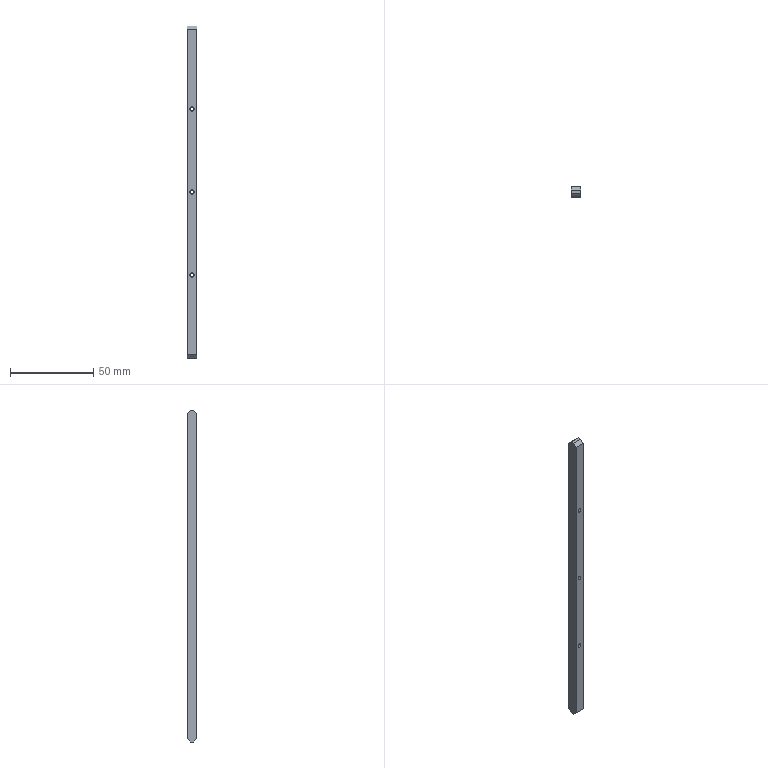Part | SolidWorks | features 3DProfileFeature 1, Chamfer 1, Extrusion 1, HoleWzd 1 | 1 solid | 16 faces | box 6 x 6 x 200 mm | volume 7064 mm3 | plane 10 | cylinder 6 | commonest cylinder face diameters 2.5 x6
STEP:
#1=CARTESIAN_POINT('',(0.,-3.,48.75));
#2=VERTEX_POINT('',#1);
#3=CARTESIAN_POINT('',(0.,-3.,51.25));
#4=VERTEX_POINT('',#3);
#5=CARTESIAN_POINT('',(0.,-3.,50.));
#6=DIRECTION('',(0.,1.,0.));
#7=DIRECTION('',(0.,0.,1.));
#8=AXIS2_PLACEMENT_3D('',#5,#6,#7);
#9=CIRCLE('',#8,1.25);
#10=EDGE_CURVE('',#2,#4,#9,.T.);
#11=ORIENTED_EDGE('',*,*,#10,.F.);
#12=CARTESIAN_POINT('',(0.,3.,48.75));
#13=VERTEX_POINT('',#12);
#14=CARTESIAN_POINT('',(0.,3.,48.75));
#15=DIRECTION('',(0.,1.,0.));
#16=VECTOR('',#15,1000.);
#17=LINE('',#14,#16);
#18=EDGE_CURVE('',#2,#13,#17,.T.);
#19=ORIENTED_EDGE('',*,*,#18,.T.);
#20=CARTESIAN_POINT('',(0.,3.,51.25));
#21=VERTEX_POINT('',#20);
#22=CARTESIAN_POINT('',(0.,3.,50.));
#23=DIRECTION('',(0.,1.,0.));
#24=DIRECTION('',(0.,0.,1.));
#25=AXIS2_PLACEMENT_3D('',#22,#23,#24);
#26=CIRCLE('',#25,1.25);
#27=EDGE_CURVE('',#13,#21,#26,.T.);
#28=ORIENTED_EDGE('',*,*,#27,.T.);
#29=CARTESIAN_POINT('',(0.,3.,51.25));
#30=DIRECTION('',(0.,1.,0.));
#31=VECTOR('',#30,1000.);
#32=LINE('',#29,#31);
#33=EDGE_CURVE('',#4,#21,#32,.T.);
#34=ORIENTED_EDGE('',*,*,#33,.F.);
#35=EDGE_LOOP('',(#11,#19,#28,#34));
#36=FACE_OUTER_BOUND('',#35,.T.);
#37=CARTESIAN_POINT('',(0.,3.,50.));
#38=DIRECTION('',(0.,1.,0.));
#39=DIRECTION('',(0.,0.,1.));
#40=AXIS2_PLACEMENT_3D('',#37,#38,#39);
#41=CYLINDRICAL_SURFACE('',#40,1.25);
#42=ADVANCED_FACE('',(#36),#41,.F.);
#43=CARTESIAN_POINT('',(0.,-3.,98.75));
#44=VERTEX_POINT('',#43);
#45=CARTESIAN_POINT('',(0.,-3.,101.25));
#46=VERTEX_POINT('',#45);
#47=CARTESIAN_POINT('',(0.,-3.,100.));
#48=DIRECTION('',(0.,1.,0.));
#49=DIRECTION('',(0.,0.,1.));
#50=AXIS2_PLACEMENT_3D('',#47,#48,#49);
#51=CIRCLE('',#50,1.25);
#52=EDGE_CURVE('',#44,#46,#51,.T.);
#53=ORIENTED_EDGE('',*,*,#52,.F.);
#54=CARTESIAN_POINT('',(0.,3.,98.75));
#55=VERTEX_POINT('',#54);
#56=CARTESIAN_POINT('',(0.,3.,98.75));
#57=DIRECTION('',(0.,1.,0.));
#58=VECTOR('',#57,1000.);
#59=LINE('',#56,#58);
#60=EDGE_CURVE('',#44,#55,#59,.T.);
#61=ORIENTED_EDGE('',*,*,#60,.T.);
#62=CARTESIAN_POINT('',(0.,3.,101.25));
#63=VERTEX_POINT('',#62);
#64=CARTESIAN_POINT('',(0.,3.,100.));
#65=DIRECTION('',(0.,1.,0.));
#66=DIRECTION('',(0.,0.,1.));
#67=AXIS2_PLACEMENT_3D('',#64,#65,#66);
#68=CIRCLE('',#67,1.25);
#69=EDGE_CURVE('',#55,#63,#68,.T.);
#70=ORIENTED_EDGE('',*,*,#69,.T.);
#71=CARTESIAN_POINT('',(0.,3.,101.25));
#72=DIRECTION('',(0.,1.,0.));
#73=VECTOR('',#72,1000.);
#74=LINE('',#71,#73);
#75=EDGE_CURVE('',#46,#63,#74,.T.);
#76=ORIENTED_EDGE('',*,*,#75,.F.);
#77=EDGE_LOOP('',(#53,#61,#70,#76));
#78=FACE_OUTER_BOUND('',#77,.T.);
#79=CARTESIAN_POINT('',(0.,3.,100.));
#80=DIRECTION('',(0.,1.,0.));
#81=DIRECTION('',(0.,0.,1.));
#82=AXIS2_PLACEMENT_3D('',#79,#80,#81);
#83=CYLINDRICAL_SURFACE('',#82,1.25);
#84=ADVANCED_FACE('',(#78),#83,.F.);
#85=CARTESIAN_POINT('',(0.,-3.,148.75));
#86=VERTEX_POINT('',#85);
#87=CARTESIAN_POINT('',(0.,-3.,151.25));
#88=VERTEX_POINT('',#87);
#89=CARTESIAN_POINT('',(0.,-3.,150.));
#90=DIRECTION('',(0.,1.,0.));
#91=DIRECTION('',(0.,0.,1.));
#92=AXIS2_PLACEMENT_3D('',#89,#90,#91);
#93=CIRCLE('',#92,1.25);
#94=EDGE_CURVE('',#86,#88,#93,.T.);
#95=ORIENTED_EDGE('',*,*,#94,.F.);
#96=CARTESIAN_POINT('',(0.,3.,148.75));
#97=VERTEX_POINT('',#96);
#98=CARTESIAN_POINT('',(0.,3.,148.75));
#99=DIRECTION('',(0.,1.,0.));
#100=VECTOR('',#99,1000.);
#101=LINE('',#98,#100);
#102=EDGE_CURVE('',#86,#97,#101,.T.);
#103=ORIENTED_EDGE('',*,*,#102,.T.);
#104=CARTESIAN_POINT('',(0.,3.,151.25));
#105=VERTEX_POINT('',#104);
#106=CARTESIAN_POINT('',(0.,3.,150.));
#107=DIRECTION('',(0.,1.,0.));
#108=DIRECTION('',(0.,0.,1.));
#109=AXIS2_PLACEMENT_3D('',#106,#107,#108);
#110=CIRCLE('',#109,1.25);
#111=EDGE_CURVE('',#97,#105,#110,.T.);
#112=ORIENTED_EDGE('',*,*,#111,.T.);
#113=CARTESIAN_POINT('',(0.,3.,151.25));
#114=DIRECTION('',(0.,1.,0.));
#115=VECTOR('',#114,1000.);
#116=LINE('',#113,#115);
#117=EDGE_CURVE('',#88,#105,#116,.T.);
#118=ORIENTED_EDGE('',*,*,#117,.F.);
#119=EDGE_LOOP('',(#95,#103,#112,#118));
#120=FACE_OUTER_BOUND('',#119,.T.);
#121=CARTESIAN_POINT('',(0.,3.,150.));
#122=DIRECTION('',(0.,1.,0.));
#123=DIRECTION('',(0.,0.,1.));
#124=AXIS2_PLACEMENT_3D('',#121,#122,#123);
#125=CYLINDRICAL_SURFACE('',#124,1.25);
#126=ADVANCED_FACE('',(#120),#125,.F.);
#127=CARTESIAN_POINT('',(3.,-3.,198.));
#128=VERTEX_POINT('',#127);
#129=CARTESIAN_POINT('',(3.,-3.,2.));
#130=VERTEX_POINT('',#129);
#131=CARTESIAN_POINT('',(3.,-3.,200.));
#132=DIRECTION('',(0.,0.,-1.));
#133=VECTOR('',#132,1000.);
#134=LINE('',#131,#133);
#135=EDGE_CURVE('',#128,#130,#134,.T.);
#136=ORIENTED_EDGE('',*,*,#135,.T.);
#137=CARTESIAN_POINT('',(3.,-1.,0.));
#138=VERTEX_POINT('',#137);
#139=CARTESIAN_POINT('',(3.,-3.,2.));
#140=DIRECTION('',(0.,0.7071,-0.7071));
#141=VECTOR('',#140,1000.);
#142=LINE('',#139,#141);
#143=EDGE_CURVE('',#130,#138,#142,.T.);
#144=ORIENTED_EDGE('',*,*,#143,.T.);
#145=CARTESIAN_POINT('',(3.,1.,0.));
#146=VERTEX_POINT('',#145);
#147=CARTESIAN_POINT('',(3.,3.,0.));
#148=DIRECTION('',(0.,1.,0.));
#149=VECTOR('',#148,1000.);
#150=LINE('',#147,#149);
#151=EDGE_CURVE('',#138,#146,#150,.T.);
#152=ORIENTED_EDGE('',*,*,#151,.T.);
#153=CARTESIAN_POINT('',(3.,3.,2.));
#154=VERTEX_POINT('',#153);
#155=CARTESIAN_POINT('',(3.,3.,2.));
#156=DIRECTION('',(0.,0.7071,0.7071));
#157=VECTOR('',#156,1000.);
#158=LINE('',#155,#157);
#159=EDGE_CURVE('',#146,#154,#158,.T.);
#160=ORIENTED_EDGE('',*,*,#159,.T.);
#161=CARTESIAN_POINT('',(3.,3.,198.));
#162=VERTEX_POINT('',#161);
#163=CARTESIAN_POINT('',(3.,3.,200.));
#164=DIRECTION('',(0.,0.,-1.));
#165=VECTOR('',#164,1000.);
#166=LINE('',#163,#165);
#167=EDGE_CURVE('',#162,#154,#166,.T.);
#168=ORIENTED_EDGE('',*,*,#167,.F.);
#169=CARTESIAN_POINT('',(3.,1.,200.));
#170=VERTEX_POINT('',#169);
#171=CARTESIAN_POINT('',(3.,1.,200.));
#172=DIRECTION('',(0.,-0.7071,0.7071));
#173=VECTOR('',#172,1000.);
#174=LINE('',#171,#173);
#175=EDGE_CURVE('',#162,#170,#174,.T.);
#176=ORIENTED_EDGE('',*,*,#175,.T.);
#177=CARTESIAN_POINT('',(3.,-1.,200.));
#178=VERTEX_POINT('',#177);
#179=CARTESIAN_POINT('',(3.,3.,200.));
#180=DIRECTION('',(0.,1.,0.));
#181=VECTOR('',#180,1000.);
#182=LINE('',#179,#181);
#183=EDGE_CURVE('',#178,#170,#182,.T.);
#184=ORIENTED_EDGE('',*,*,#183,.F.);
#185=CARTESIAN_POINT('',(3.,-1.,200.));
#186=DIRECTION('',(0.,-0.7071,-0.7071));
#187=VECTOR('',#186,1000.);
#188=LINE('',#185,#187);
#189=EDGE_CURVE('',#178,#128,#188,.T.);
#190=ORIENTED_EDGE('',*,*,#189,.T.);
#191=EDGE_LOOP('',(#136,#144,#152,#160,#168,#176,#184,#190));
#192=FACE_OUTER_BOUND('',#191,.T.);
#193=CARTESIAN_POINT('',(3.,3.,200.));
#194=DIRECTION('',(-1.,0.,0.));
#195=DIRECTION('',(0.,-1.,0.));
#196=AXIS2_PLACEMENT_3D('',#193,#194,#195);
#197=PLANE('',#196);
#198=ADVANCED_FACE('',(#192),#197,.F.);
#199=CARTESIAN_POINT('',(0.,3.,50.));
#200=DIRECTION('',(0.,1.,0.));
#201=DIRECTION('',(0.,0.,1.));
#202=AXIS2_PLACEMENT_3D('',#199,#200,#201);
#203=CIRCLE('',#202,1.25);
#204=EDGE_CURVE('',#21,#13,#203,.T.);
#205=ORIENTED_EDGE('',*,*,#204,.F.);
#206=ORIENTED_EDGE('',*,*,#27,.F.);
#207=EDGE_LOOP('',(#205,#206));
#208=FACE_BOUND('',#207,.T.);
#209=CARTESIAN_POINT('',(0.,3.,100.));
#210=DIRECTION('',(0.,1.,0.));
#211=DIRECTION('',(0.,0.,1.));
#212=AXIS2_PLACEMENT_3D('',#209,#210,#211);
#213=CIRCLE('',#212,1.25);
#214=EDGE_CURVE('',#63,#55,#213,.T.);
#215=ORIENTED_EDGE('',*,*,#214,.F.);
#216=ORIENTED_EDGE('',*,*,#69,.F.);
#217=EDGE_LOOP('',(#215,#216));
#218=FACE_BOUND('',#217,.T.);
#219=CARTESIAN_POINT('',(0.,3.,150.));
#220=DIRECTION('',(0.,1.,0.));
#221=DIRECTION('',(0.,0.,1.));
#222=AXIS2_PLACEMENT_3D('',#219,#220,#221);
#223=CIRCLE('',#222,1.25);
#224=EDGE_CURVE('',#105,#97,#223,.T.);
#225=ORIENTED_EDGE('',*,*,#224,.F.);
#226=ORIENTED_EDGE('',*,*,#111,.F.);
#227=EDGE_LOOP('',(#225,#226));
#228=FACE_BOUND('',#227,.T.);
#229=ORIENTED_EDGE('',*,*,#167,.T.);
#230=CARTESIAN_POINT('',(-3.,3.,2.));
#231=VERTEX_POINT('',#230);
#232=CARTESIAN_POINT('',(-3.,3.,2.));
#233=DIRECTION('',(-1.,0.,0.));
#234=VECTOR('',#233,1000.);
#235=LINE('',#232,#234);
#236=EDGE_CURVE('',#154,#231,#235,.T.);
#237=ORIENTED_EDGE('',*,*,#236,.T.);
#238=CARTESIAN_POINT('',(-3.,3.,198.));
#239=VERTEX_POINT('',#238);
#240=CARTESIAN_POINT('',(-3.,3.,200.));
#241=DIRECTION('',(0.,0.,-1.));
#242=VECTOR('',#241,1000.);
#243=LINE('',#240,#242);
#244=EDGE_CURVE('',#239,#231,#243,.T.);
#245=ORIENTED_EDGE('',*,*,#244,.F.);
#246=CARTESIAN_POINT('',(3.,3.,198.));
#247=DIRECTION('',(1.,0.,0.));
#248=VECTOR('',#247,1000.);
#249=LINE('',#246,#248);
#250=EDGE_CURVE('',#239,#162,#249,.T.);
#251=ORIENTED_EDGE('',*,*,#250,.T.);
#252=EDGE_LOOP('',(#229,#237,#245,#251));
#253=FACE_OUTER_BOUND('',#252,.T.);
#254=CARTESIAN_POINT('',(-3.,3.,200.));
#255=DIRECTION('',(0.,-1.,0.));
#256=DIRECTION('',(0.,0.,-1.));
#257=AXIS2_PLACEMENT_3D('',#254,#255,#256);
#258=PLANE('',#257);
#259=ADVANCED_FACE('',(#208,#218,#228,#253),#258,.F.);
#260=CARTESIAN_POINT('',(-3.,1.,0.));
#261=VERTEX_POINT('',#260);
#262=CARTESIAN_POINT('',(-3.,-1.,0.));
#263=VERTEX_POINT('',#262);
#264=CARTESIAN_POINT('',(-3.,3.,0.));
#265=DIRECTION('',(0.,-1.,0.));
#266=VECTOR('',#265,1000.);
#267=LINE('',#264,#266);
#268=EDGE_CURVE('',#261,#263,#267,.T.);
#269=ORIENTED_EDGE('',*,*,#268,.T.);
#270=CARTESIAN_POINT('',(-3.,-3.,2.));
#271=VERTEX_POINT('',#270);
#272=CARTESIAN_POINT('',(-3.,-3.,2.));
#273=DIRECTION('',(0.,-0.7071,0.7071));
#274=VECTOR('',#273,1000.);
#275=LINE('',#272,#274);
#276=EDGE_CURVE('',#263,#271,#275,.T.);
#277=ORIENTED_EDGE('',*,*,#276,.T.);
#278=CARTESIAN_POINT('',(-3.,-3.,198.));
#279=VERTEX_POINT('',#278);
#280=CARTESIAN_POINT('',(-3.,-3.,200.));
#281=DIRECTION('',(0.,0.,-1.));
#282=VECTOR('',#281,1000.);
#283=LINE('',#280,#282);
#284=EDGE_CURVE('',#279,#271,#283,.T.);
#285=ORIENTED_EDGE('',*,*,#284,.F.);
#286=CARTESIAN_POINT('',(-3.,-1.,200.));
#287=VERTEX_POINT('',#286);
#288=CARTESIAN_POINT('',(-3.,-1.,200.));
#289=DIRECTION('',(0.,0.7071,0.7071));
#290=VECTOR('',#289,1000.);
#291=LINE('',#288,#290);
#292=EDGE_CURVE('',#279,#287,#291,.T.);
#293=ORIENTED_EDGE('',*,*,#292,.T.);
#294=CARTESIAN_POINT('',(-3.,1.,200.));
#295=VERTEX_POINT('',#294);
#296=CARTESIAN_POINT('',(-3.,3.,200.));
#297=DIRECTION('',(0.,-1.,0.));
#298=VECTOR('',#297,1000.);
#299=LINE('',#296,#298);
#300=EDGE_CURVE('',#295,#287,#299,.T.);
#301=ORIENTED_EDGE('',*,*,#300,.F.);
#302=CARTESIAN_POINT('',(-3.,1.,200.));
#303=DIRECTION('',(0.,0.7071,-0.7071));
#304=VECTOR('',#303,1000.);
#305=LINE('',#302,#304);
#306=EDGE_CURVE('',#295,#239,#305,.T.);
#307=ORIENTED_EDGE('',*,*,#306,.T.);
#308=ORIENTED_EDGE('',*,*,#244,.T.);
#309=CARTESIAN_POINT('',(-3.,3.,2.));
#310=DIRECTION('',(0.,-0.7071,-0.7071));
#311=VECTOR('',#310,1000.);
#312=LINE('',#309,#311);
#313=EDGE_CURVE('',#231,#261,#312,.T.);
#314=ORIENTED_EDGE('',*,*,#313,.T.);
#315=EDGE_LOOP('',(#269,#277,#285,#293,#301,#307,#308,#314));
#316=FACE_OUTER_BOUND('',#315,.T.);
#317=CARTESIAN_POINT('',(-3.,3.,200.));
#318=DIRECTION('',(1.,0.,0.));
#319=DIRECTION('',(0.,1.,0.));
#320=AXIS2_PLACEMENT_3D('',#317,#318,#319);
#321=PLANE('',#320);
#322=ADVANCED_FACE('',(#316),#321,.F.);
#323=CARTESIAN_POINT('',(0.,-3.,50.));
#324=DIRECTION('',(0.,1.,0.));
#325=DIRECTION('',(0.,0.,1.));
#326=AXIS2_PLACEMENT_3D('',#323,#324,#325);
#327=CIRCLE('',#326,1.25);
#328=EDGE_CURVE('',#4,#2,#327,.T.);
#329=ORIENTED_EDGE('',*,*,#328,.T.);
#330=ORIENTED_EDGE('',*,*,#10,.T.);
#331=EDGE_LOOP('',(#329,#330));
#332=FACE_BOUND('',#331,.T.);
#333=CARTESIAN_POINT('',(0.,-3.,100.));
#334=DIRECTION('',(0.,1.,0.));
#335=DIRECTION('',(0.,0.,1.));
#336=AXIS2_PLACEMENT_3D('',#333,#334,#335);
#337=CIRCLE('',#336,1.25);
#338=EDGE_CURVE('',#46,#44,#337,.T.);
#339=ORIENTED_EDGE('',*,*,#338,.T.);
#340=ORIENTED_EDGE('',*,*,#52,.T.);
#341=EDGE_LOOP('',(#339,#340));
#342=FACE_BOUND('',#341,.T.);
#343=CARTESIAN_POINT('',(0.,-3.,150.));
#344=DIRECTION('',(0.,1.,0.));
#345=DIRECTION('',(0.,0.,1.));
#346=AXIS2_PLACEMENT_3D('',#343,#344,#345);
#347=CIRCLE('',#346,1.25);
#348=EDGE_CURVE('',#88,#86,#347,.T.);
#349=ORIENTED_EDGE('',*,*,#348,.T.);
#350=ORIENTED_EDGE('',*,*,#94,.T.);
#351=EDGE_LOOP('',(#349,#350));
#352=FACE_BOUND('',#351,.T.);
#353=ORIENTED_EDGE('',*,*,#284,.T.);
#354=CARTESIAN_POINT('',(-3.,-3.,2.));
#355=DIRECTION('',(1.,0.,0.));
#356=VECTOR('',#355,1000.);
#357=LINE('',#354,#356);
#358=EDGE_CURVE('',#271,#130,#357,.T.);
#359=ORIENTED_EDGE('',*,*,#358,.T.);
#360=ORIENTED_EDGE('',*,*,#135,.F.);
#361=CARTESIAN_POINT('',(-3.,-3.,198.));
#362=DIRECTION('',(-1.,0.,0.));
#363=VECTOR('',#362,1000.);
#364=LINE('',#361,#363);
#365=EDGE_CURVE('',#128,#279,#364,.T.);
#366=ORIENTED_EDGE('',*,*,#365,.T.);
#367=EDGE_LOOP('',(#353,#359,#360,#366));
#368=FACE_OUTER_BOUND('',#367,.T.);
#369=CARTESIAN_POINT('',(-3.,-3.,200.));
#370=DIRECTION('',(0.,1.,0.));
#371=DIRECTION('',(0.,0.,1.));
#372=AXIS2_PLACEMENT_3D('',#369,#370,#371);
#373=PLANE('',#372);
#374=ADVANCED_FACE('',(#332,#342,#352,#368),#373,.F.);
#375=ORIENTED_EDGE('',*,*,#300,.T.);
#376=CARTESIAN_POINT('',(3.,-1.,200.));
#377=DIRECTION('',(1.,0.,0.));
#378=VECTOR('',#377,1000.);
#379=LINE('',#376,#378);
#380=EDGE_CURVE('',#287,#178,#379,.T.);
#381=ORIENTED_EDGE('',*,*,#380,.T.);
#382=ORIENTED_EDGE('',*,*,#183,.T.);
#383=CARTESIAN_POINT('',(-3.,1.,200.));
#384=DIRECTION('',(-1.,0.,0.));
#385=VECTOR('',#384,1000.);
#386=LINE('',#383,#385);
#387=EDGE_CURVE('',#170,#295,#386,.T.);
#388=ORIENTED_EDGE('',*,*,#387,.T.);
#389=EDGE_LOOP('',(#375,#381,#382,#388));
#390=FACE_OUTER_BOUND('',#389,.T.);
#391=CARTESIAN_POINT('',(0.,0.,200.));
#392=DIRECTION('',(0.,0.,1.));
#393=DIRECTION('',(1.,0.,0.));
#394=AXIS2_PLACEMENT_3D('',#391,#392,#393);
#395=PLANE('',#394);
#396=ADVANCED_FACE('',(#390),#395,.T.);
#397=ORIENTED_EDGE('',*,*,#151,.F.);
#398=CARTESIAN_POINT('',(0.,-1.,0.));
#399=DIRECTION('',(-1.,0.,0.));
#400=VECTOR('',#399,1000.);
#401=LINE('',#398,#400);
#402=EDGE_CURVE('',#138,#263,#401,.T.);
#403=ORIENTED_EDGE('',*,*,#402,.T.);
#404=ORIENTED_EDGE('',*,*,#268,.F.);
#405=CARTESIAN_POINT('',(0.,1.,0.));
#406=DIRECTION('',(1.,0.,0.));
#407=VECTOR('',#406,1000.);
#408=LINE('',#405,#407);
#409=EDGE_CURVE('',#261,#146,#408,.T.);
#410=ORIENTED_EDGE('',*,*,#409,.T.);
#411=EDGE_LOOP('',(#397,#403,#404,#410));
#412=FACE_OUTER_BOUND('',#411,.T.);
#413=CARTESIAN_POINT('',(0.,0.,0.));
#414=DIRECTION('',(0.,0.,1.));
#415=DIRECTION('',(1.,0.,0.));
#416=AXIS2_PLACEMENT_3D('',#413,#414,#415);
#417=PLANE('',#416);
#418=ADVANCED_FACE('',(#412),#417,.F.);
#419=ORIENTED_EDGE('',*,*,#102,.F.);
#420=ORIENTED_EDGE('',*,*,#348,.F.);
#421=ORIENTED_EDGE('',*,*,#117,.T.);
#422=ORIENTED_EDGE('',*,*,#224,.T.);
#423=EDGE_LOOP('',(#419,#420,#421,#422));
#424=FACE_OUTER_BOUND('',#423,.T.);
#425=CARTESIAN_POINT('',(0.,3.,150.));
#426=DIRECTION('',(0.,1.,0.));
#427=DIRECTION('',(0.,0.,1.));
#428=AXIS2_PLACEMENT_3D('',#425,#426,#427);
#429=CYLINDRICAL_SURFACE('',#428,1.25);
#430=ADVANCED_FACE('',(#424),#429,.F.);
#431=ORIENTED_EDGE('',*,*,#60,.F.);
#432=ORIENTED_EDGE('',*,*,#338,.F.);
#433=ORIENTED_EDGE('',*,*,#75,.T.);
#434=ORIENTED_EDGE('',*,*,#214,.T.);
#435=EDGE_LOOP('',(#431,#432,#433,#434));
#436=FACE_OUTER_BOUND('',#435,.T.);
#437=CARTESIAN_POINT('',(0.,3.,100.));
#438=DIRECTION('',(0.,1.,0.));
#439=DIRECTION('',(0.,0.,1.));
#440=AXIS2_PLACEMENT_3D('',#437,#438,#439);
#441=CYLINDRICAL_SURFACE('',#440,1.25);
#442=ADVANCED_FACE('',(#436),#441,.F.);
#443=ORIENTED_EDGE('',*,*,#18,.F.);
#444=ORIENTED_EDGE('',*,*,#328,.F.);
#445=ORIENTED_EDGE('',*,*,#33,.T.);
#446=ORIENTED_EDGE('',*,*,#204,.T.);
#447=EDGE_LOOP('',(#443,#444,#445,#446));
#448=FACE_OUTER_BOUND('',#447,.T.);
#449=CARTESIAN_POINT('',(0.,3.,50.));
#450=DIRECTION('',(0.,1.,0.));
#451=DIRECTION('',(0.,0.,1.));
#452=AXIS2_PLACEMENT_3D('',#449,#450,#451);
#453=CYLINDRICAL_SURFACE('',#452,1.25);
#454=ADVANCED_FACE('',(#448),#453,.F.);
#455=ORIENTED_EDGE('',*,*,#276,.F.);
#456=ORIENTED_EDGE('',*,*,#402,.F.);
#457=ORIENTED_EDGE('',*,*,#143,.F.);
#458=ORIENTED_EDGE('',*,*,#358,.F.);
#459=EDGE_LOOP('',(#455,#456,#457,#458));
#460=FACE_OUTER_BOUND('',#459,.T.);
#461=CARTESIAN_POINT('',(-3.,-3.,2.));
#462=DIRECTION('',(0.,0.7071,0.7071));
#463=DIRECTION('',(1.,0.,0.));
#464=AXIS2_PLACEMENT_3D('',#461,#462,#463);
#465=PLANE('',#464);
#466=ADVANCED_FACE('',(#460),#465,.F.);
#467=ORIENTED_EDGE('',*,*,#159,.F.);
#468=ORIENTED_EDGE('',*,*,#409,.F.);
#469=ORIENTED_EDGE('',*,*,#313,.F.);
#470=ORIENTED_EDGE('',*,*,#236,.F.);
#471=EDGE_LOOP('',(#467,#468,#469,#470));
#472=FACE_OUTER_BOUND('',#471,.T.);
#473=CARTESIAN_POINT('',(-3.,3.,2.));
#474=DIRECTION('',(0.,-0.7071,0.7071));
#475=DIRECTION('',(-1.,0.,0.));
#476=AXIS2_PLACEMENT_3D('',#473,#474,#475);
#477=PLANE('',#476);
#478=ADVANCED_FACE('',(#472),#477,.F.);
#479=ORIENTED_EDGE('',*,*,#292,.F.);
#480=ORIENTED_EDGE('',*,*,#365,.F.);
#481=ORIENTED_EDGE('',*,*,#189,.F.);
#482=ORIENTED_EDGE('',*,*,#380,.F.);
#483=EDGE_LOOP('',(#479,#480,#481,#482));
#484=FACE_OUTER_BOUND('',#483,.T.);
#485=CARTESIAN_POINT('',(0.,-1.,200.));
#486=DIRECTION('',(0.,-0.7071,0.7071));
#487=DIRECTION('',(-1.,0.,0.));
#488=AXIS2_PLACEMENT_3D('',#485,#486,#487);
#489=PLANE('',#488);
#490=ADVANCED_FACE('',(#484),#489,.T.);
#491=ORIENTED_EDGE('',*,*,#175,.F.);
#492=ORIENTED_EDGE('',*,*,#250,.F.);
#493=ORIENTED_EDGE('',*,*,#306,.F.);
#494=ORIENTED_EDGE('',*,*,#387,.F.);
#495=EDGE_LOOP('',(#491,#492,#493,#494));
#496=FACE_OUTER_BOUND('',#495,.T.);
#497=CARTESIAN_POINT('',(0.,1.,200.));
#498=DIRECTION('',(0.,0.7071,0.7071));
#499=DIRECTION('',(1.,0.,0.));
#500=AXIS2_PLACEMENT_3D('',#497,#498,#499);
#501=PLANE('',#500);
#502=ADVANCED_FACE('',(#496),#501,.T.);
#503=CLOSED_SHELL('',(#42,#84,#126,#198,#259,#322,#374,#396,#418,#430,#442,#454,#466,#478,#490,#502));
#504=MANIFOLD_SOLID_BREP('',#503);
#505=CARTESIAN_POINT('',(0.,0.,0.));
#506=DIRECTION('',(0.,0.,1.));
#507=DIRECTION('',(1.,0.,0.));
#508=AXIS2_PLACEMENT_3D('',#505,#506,#507);
#509=(LENGTH_UNIT()NAMED_UNIT(*)SI_UNIT(.MILLI.,.METRE.));
#510=UNCERTAINTY_MEASURE_WITH_UNIT(LENGTH_MEASURE(0.00001),#509,'','');
#511=(NAMED_UNIT(*)PLANE_ANGLE_UNIT()SI_UNIT($,.RADIAN.));
#512=(NAMED_UNIT(*)SI_UNIT($,.STERADIAN.)SOLID_ANGLE_UNIT());
#513=(GEOMETRIC_REPRESENTATION_CONTEXT(3)GLOBAL_UNCERTAINTY_ASSIGNED_CONTEXT((#510))GLOBAL_UNIT_ASSIGNED_CONTEXT((#509,#511,#512))REPRESENTATION_CONTEXT('',''));
#514=ADVANCED_BREP_SHAPE_REPRESENTATION('',(#504,#508),#513);